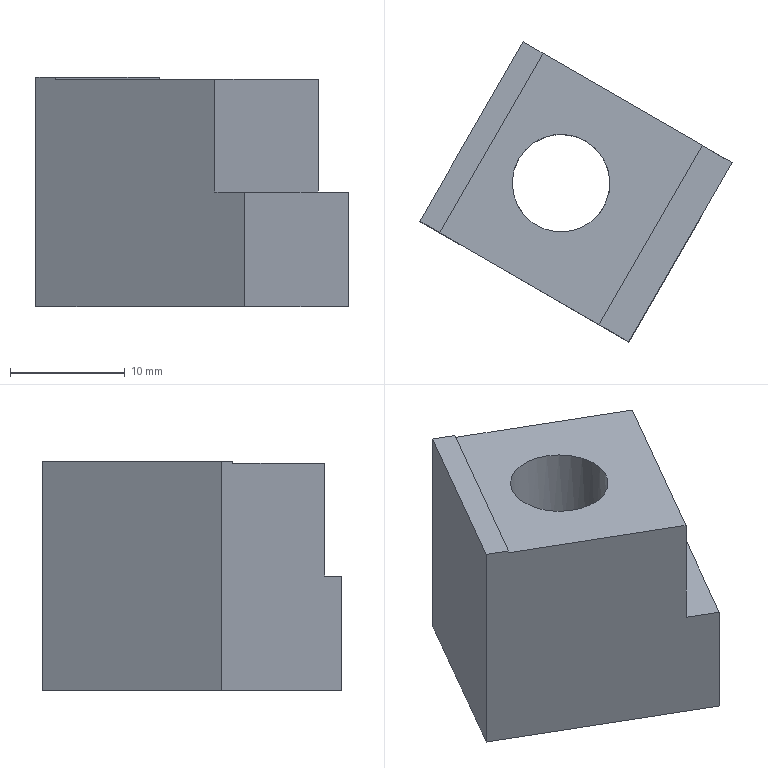Part | NX | features solid 2 | 1 solid | 104 faces | box 27.187 x 26.088 x 20 mm | volume 4669 mm3 | plane 80 | spline 22 | cylinder 2 | commonest cylinder face diameters 8.5 x1 14 x1